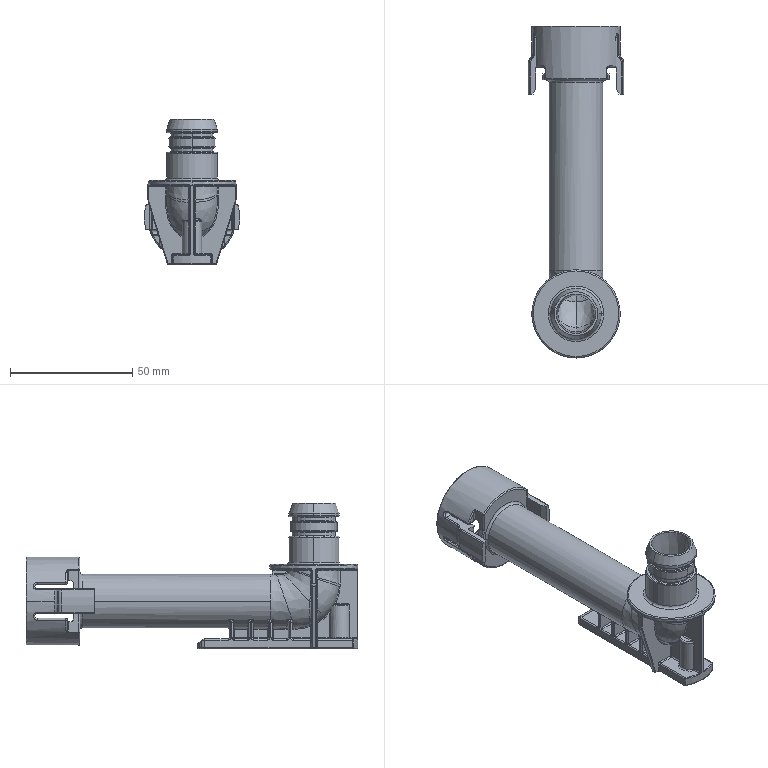Part | STEP file | ZXW722-L-20 | 1 solid | 1005 faces | box 39 x 135.5 x 59.4 mm | volume 32413 mm3 | cylinder 368 | torus 176 | spline 171 | plane 165 | sphere 107 | cone 18 | commonest cylinder face diameters 1 x304 2 x12 0.6 x11 4 x7 36 x6 17.6 x4